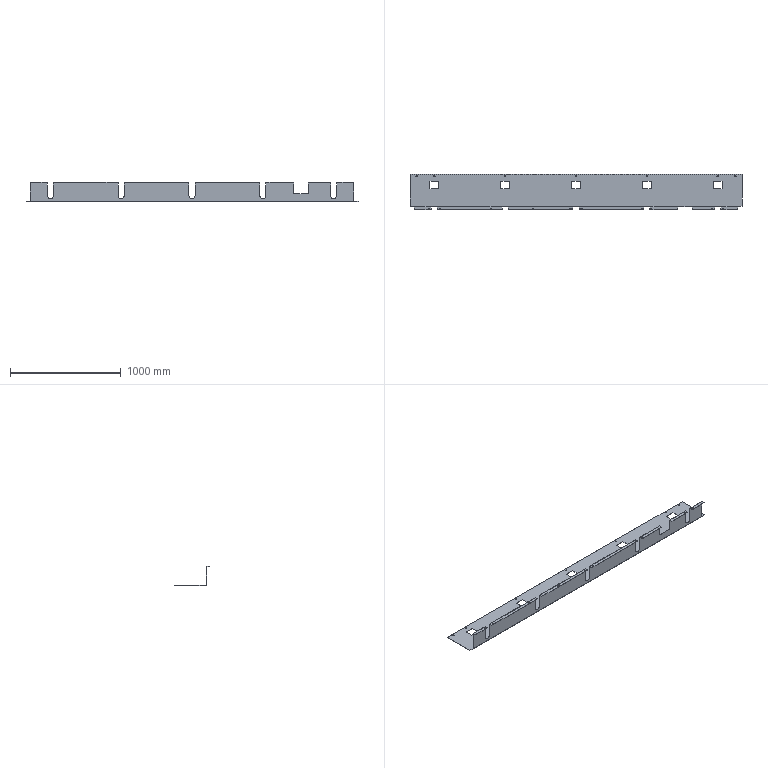Part | SolidWorks | features BaseBody 1 | 1 solid | 167 faces | box 3000 x 321 x 172 mm | volume 2714795 mm3 | plane 95 | cylinder 72 | commonest cylinder face diameters 7 x45 4 x8 8 x8 55 x5 13 x4 20 x2